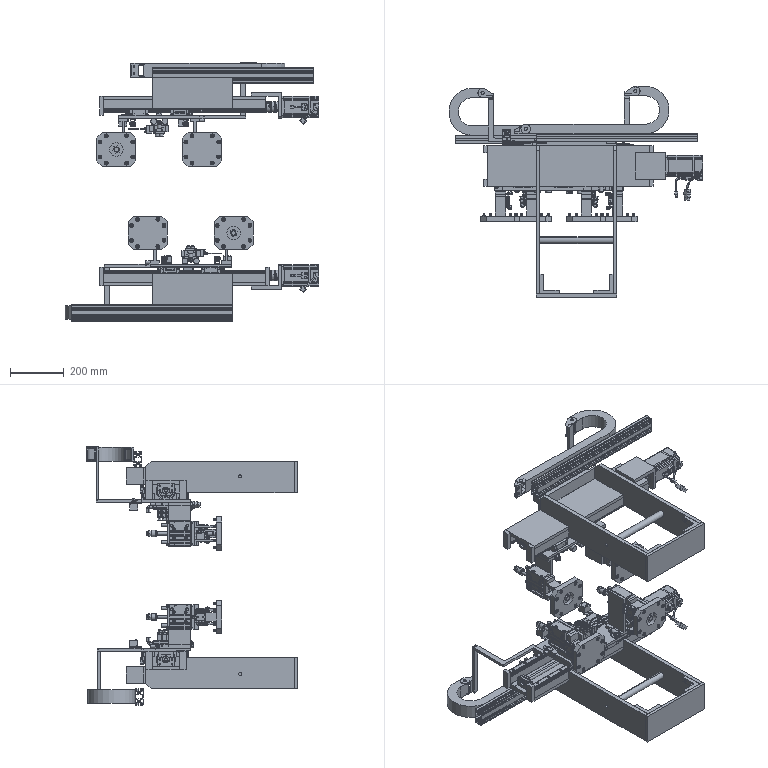Part | SolidWorks | features CompositeCurve 32, InContextFeatHolder 3 | 332 solids | 19692 faces | volume 21572641 mm3 | plane 9775 | cylinder 5505 | cone 2972 | spline 1264 | torus 120 | sphere 56 | commonest cylinder face diameters 8 x312 6 x274 2 x254 4 x244 1 x174 9 x162